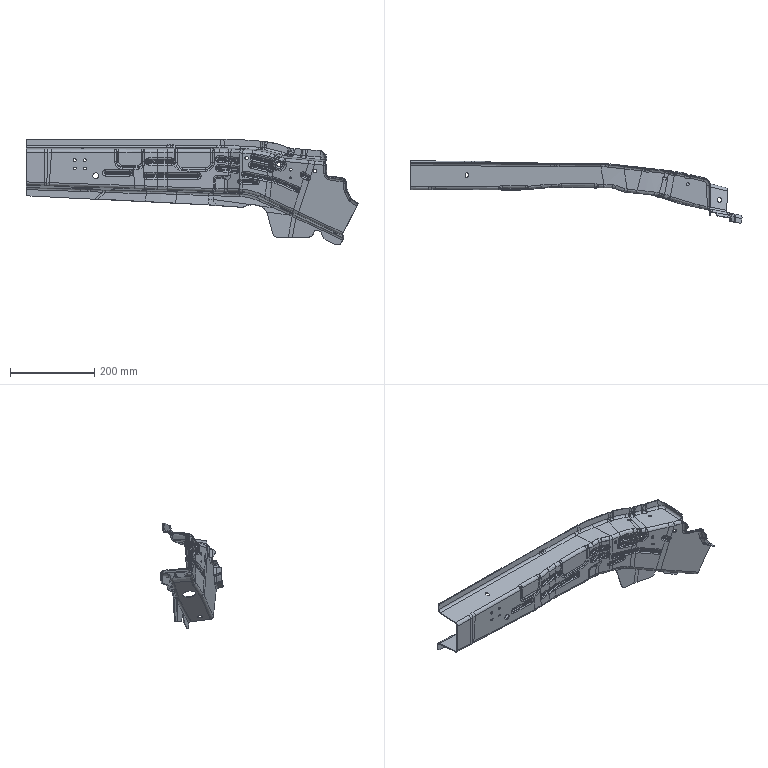Part | 1 solid | 1457 faces | box 789.649 x 148.577 x 251.714 mm | volume 397464 mm3 | spline 1144 | cylinder 240 | plane 55 | other 14 | sphere 4 | commonest cylinder face diameters 10 x36 16 x30 6 x26 11 x22 12 x22 15 x22